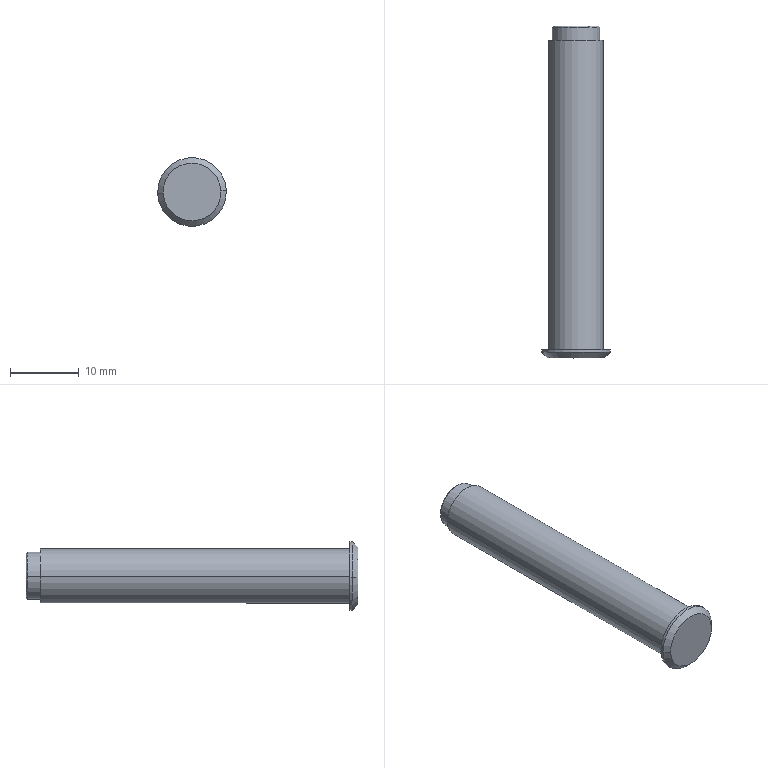Part | SolidWorks | features BaseBody 1 | 1 solid | 17 faces | box 10 x 48.303 x 10 mm | volume 2156 mm3 | cylinder 8 | plane 5 | cone 4 | commonest cylinder face diameters 5.2 x2 6.9 x2 7.9 x2 10 x2
STEP:
#1=CARTESIAN_POINT('',(-215.071,6.123,1.995));
#2=VERTEX_POINT('',#1);
#3=CARTESIAN_POINT('',(-209.875,6.123,2.179));
#4=VERTEX_POINT('',#3);
#5=CARTESIAN_POINT('',(-212.473,6.123,2.087));
#6=DIRECTION('',(0.00003827,-1.,-0.0004455));
#7=DIRECTION('',(-0.9994,-0.0000225,-0.03534));
#8=AXIS2_PLACEMENT_3D('',#5,#6,#7);
#9=CIRCLE('',#8,2.6);
#10=EDGE_CURVE('',#2,#4,#9,.T.);
#11=ORIENTED_EDGE('',*,*,#10,.F.);
#12=CARTESIAN_POINT('',(-212.473,6.123,2.087));
#13=DIRECTION('',(0.00003827,-1.,-0.0004455));
#14=DIRECTION('',(0.9994,0.0000225,0.03534));
#15=AXIS2_PLACEMENT_3D('',#12,#13,#14);
#16=CIRCLE('',#15,2.6);
#17=EDGE_CURVE('',#4,#2,#16,.T.);
#18=ORIENTED_EDGE('',*,*,#17,.F.);
#19=EDGE_LOOP('',(#11,#18));
#20=FACE_OUTER_BOUND('',#19,.T.);
#21=CARTESIAN_POINT('',(-212.473,6.123,2.087));
#22=DIRECTION('',(-0.00003827,1.,0.0004455));
#23=DIRECTION('',(0.9963,0.,0.08559));
#24=AXIS2_PLACEMENT_3D('',#21,#22,#23);
#25=PLANE('',#24);
#26=ADVANCED_FACE('',(#20),#25,.T.);
#27=ORIENTED_EDGE('',*,*,#17,.T.);
#28=CARTESIAN_POINT('',(-215.072,16.123,2.));
#29=VERTEX_POINT('',#28);
#30=CARTESIAN_POINT('',(-215.072,16.123,2.));
#31=DIRECTION('',(0.00003827,-1.,-0.0004455));
#32=VECTOR('',#31,1000.);
#33=LINE('',#30,#32);
#34=EDGE_CURVE('',#29,#2,#33,.T.);
#35=ORIENTED_EDGE('',*,*,#34,.F.);
#36=CARTESIAN_POINT('',(-209.875,16.123,2.183));
#37=VERTEX_POINT('',#36);
#38=CARTESIAN_POINT('',(-212.473,16.123,2.092));
#39=DIRECTION('',(-0.00003827,1.,0.0004455));
#40=DIRECTION('',(-0.9994,-0.0000225,-0.03534));
#41=AXIS2_PLACEMENT_3D('',#38,#39,#40);
#42=CIRCLE('',#41,2.6);
#43=EDGE_CURVE('',#29,#37,#42,.T.);
#44=ORIENTED_EDGE('',*,*,#43,.T.);
#45=CARTESIAN_POINT('',(-209.875,16.123,2.183));
#46=DIRECTION('',(0.00003827,-1.,-0.0004455));
#47=VECTOR('',#46,1000.);
#48=LINE('',#45,#47);
#49=EDGE_CURVE('',#37,#4,#48,.T.);
#50=ORIENTED_EDGE('',*,*,#49,.T.);
#51=EDGE_LOOP('',(#27,#35,#44,#50));
#52=FACE_OUTER_BOUND('',#51,.T.);
#53=CARTESIAN_POINT('',(-212.473,6.123,2.087));
#54=DIRECTION('',(-0.00003827,1.,0.0004455));
#55=DIRECTION('',(-0.9994,-0.0000225,-0.03534));
#56=AXIS2_PLACEMENT_3D('',#53,#54,#55);
#57=CYLINDRICAL_SURFACE('',#56,2.6);
#58=ADVANCED_FACE('',(#52),#57,.F.);
#59=ORIENTED_EDGE('',*,*,#49,.F.);
#60=CARTESIAN_POINT('',(-212.473,16.123,2.092));
#61=DIRECTION('',(-0.00003827,1.,0.0004455));
#62=DIRECTION('',(0.9994,0.0000225,0.03534));
#63=AXIS2_PLACEMENT_3D('',#60,#61,#62);
#64=CIRCLE('',#63,2.6);
#65=EDGE_CURVE('',#37,#29,#64,.T.);
#66=ORIENTED_EDGE('',*,*,#65,.T.);
#67=ORIENTED_EDGE('',*,*,#34,.T.);
#68=ORIENTED_EDGE('',*,*,#10,.T.);
#69=EDGE_LOOP('',(#59,#66,#67,#68));
#70=FACE_OUTER_BOUND('',#69,.T.);
#71=CARTESIAN_POINT('',(-212.473,6.123,2.087));
#72=DIRECTION('',(-0.00003827,1.,0.0004455));
#73=DIRECTION('',(-0.9994,-0.0000225,-0.03534));
#74=AXIS2_PLACEMENT_3D('',#71,#72,#73);
#75=CYLINDRICAL_SURFACE('',#74,2.6);
#76=ADVANCED_FACE('',(#70),#75,.F.);
#77=ORIENTED_EDGE('',*,*,#65,.F.);
#78=ORIENTED_EDGE('',*,*,#43,.F.);
#79=EDGE_LOOP('',(#77,#78));
#80=FACE_BOUND('',#79,.T.);
#81=CARTESIAN_POINT('',(-209.225,16.123,2.206));
#82=VERTEX_POINT('',#81);
#83=CARTESIAN_POINT('',(-215.721,16.123,1.977));
#84=VERTEX_POINT('',#83);
#85=CARTESIAN_POINT('',(-212.473,16.123,2.092));
#86=DIRECTION('',(0.00003827,-1.,-0.0004455));
#87=DIRECTION('',(0.9994,0.0000225,0.03534));
#88=AXIS2_PLACEMENT_3D('',#85,#86,#87);
#89=CIRCLE('',#88,3.25);
#90=EDGE_CURVE('',#82,#84,#89,.T.);
#91=ORIENTED_EDGE('',*,*,#90,.F.);
#92=CARTESIAN_POINT('',(-212.473,16.123,2.092));
#93=DIRECTION('',(0.00003827,-1.,-0.0004455));
#94=DIRECTION('',(-0.9994,-0.0000225,-0.03534));
#95=AXIS2_PLACEMENT_3D('',#92,#93,#94);
#96=CIRCLE('',#95,3.25);
#97=EDGE_CURVE('',#84,#82,#96,.T.);
#98=ORIENTED_EDGE('',*,*,#97,.F.);
#99=EDGE_LOOP('',(#91,#98));
#100=FACE_OUTER_BOUND('',#99,.T.);
#101=CARTESIAN_POINT('',(-212.473,16.123,2.092));
#102=DIRECTION('',(-0.00003827,1.,0.0004455));
#103=DIRECTION('',(0.9963,0.,0.08559));
#104=AXIS2_PLACEMENT_3D('',#101,#102,#103);
#105=PLANE('',#104);
#106=ADVANCED_FACE('',(#80,#100),#105,.T.);
#107=ORIENTED_EDGE('',*,*,#97,.T.);
#108=CARTESIAN_POINT('',(-209.025,15.923,2.213));
#109=VERTEX_POINT('',#108);
#110=CARTESIAN_POINT('',(-209.025,15.923,2.213));
#111=DIRECTION('',(-0.7067,0.7071,-0.02468));
#112=VECTOR('',#111,1000.);
#113=LINE('',#110,#112);
#114=EDGE_CURVE('',#109,#82,#113,.T.);
#115=ORIENTED_EDGE('',*,*,#114,.F.);
#116=CARTESIAN_POINT('',(-215.921,15.923,1.97));
#117=VERTEX_POINT('',#116);
#118=CARTESIAN_POINT('',(-212.473,15.923,2.091));
#119=DIRECTION('',(0.00003827,-1.,-0.0004455));
#120=DIRECTION('',(-0.9994,-0.0000225,-0.03534));
#121=AXIS2_PLACEMENT_3D('',#118,#119,#120);
#122=CIRCLE('',#121,3.45);
#123=EDGE_CURVE('',#117,#109,#122,.T.);
#124=ORIENTED_EDGE('',*,*,#123,.F.);
#125=CARTESIAN_POINT('',(-215.921,15.923,1.97));
#126=DIRECTION('',(0.7066,0.7071,0.02531));
#127=VECTOR('',#126,1000.);
#128=LINE('',#125,#127);
#129=EDGE_CURVE('',#117,#84,#128,.T.);
#130=ORIENTED_EDGE('',*,*,#129,.T.);
#131=EDGE_LOOP('',(#107,#115,#124,#130));
#132=FACE_OUTER_BOUND('',#131,.T.);
#133=CARTESIAN_POINT('',(-212.473,16.023,2.092));
#134=DIRECTION('',(0.00003827,-1.,-0.0004455));
#135=DIRECTION('',(0.9994,0.0000225,0.03534));
#136=AXIS2_PLACEMENT_3D('',#133,#134,#135);
#137=CONICAL_SURFACE('',#136,3.35,0.7854);
#138=ADVANCED_FACE('',(#132),#137,.T.);
#139=ORIENTED_EDGE('',*,*,#129,.F.);
#140=CARTESIAN_POINT('',(-212.473,15.923,2.091));
#141=DIRECTION('',(0.00003827,-1.,-0.0004455));
#142=DIRECTION('',(0.9994,0.0000225,0.03534));
#143=AXIS2_PLACEMENT_3D('',#140,#141,#142);
#144=CIRCLE('',#143,3.45);
#145=EDGE_CURVE('',#109,#117,#144,.T.);
#146=ORIENTED_EDGE('',*,*,#145,.F.);
#147=ORIENTED_EDGE('',*,*,#114,.T.);
#148=ORIENTED_EDGE('',*,*,#90,.T.);
#149=EDGE_LOOP('',(#139,#146,#147,#148));
#150=FACE_OUTER_BOUND('',#149,.T.);
#151=CARTESIAN_POINT('',(-212.473,16.023,2.092));
#152=DIRECTION('',(0.00003827,-1.,-0.0004455));
#153=DIRECTION('',(0.9994,0.0000225,0.03534));
#154=AXIS2_PLACEMENT_3D('',#151,#152,#153);
#155=CONICAL_SURFACE('',#154,3.35,0.7854);
#156=ADVANCED_FACE('',(#150),#155,.T.);
#157=CARTESIAN_POINT('',(-215.921,14.023,1.969));
#158=VERTEX_POINT('',#157);
#159=CARTESIAN_POINT('',(-215.921,14.023,1.969));
#160=DIRECTION('',(-0.00003827,1.,0.0004455));
#161=VECTOR('',#160,1000.);
#162=LINE('',#159,#161);
#163=EDGE_CURVE('',#158,#117,#162,.T.);
#164=ORIENTED_EDGE('',*,*,#163,.F.);
#165=CARTESIAN_POINT('',(-209.025,14.023,2.213));
#166=VERTEX_POINT('',#165);
#167=CARTESIAN_POINT('',(-212.473,14.023,2.091));
#168=DIRECTION('',(-0.00003827,1.,0.0004455));
#169=DIRECTION('',(-0.9994,-0.0000225,-0.03534));
#170=AXIS2_PLACEMENT_3D('',#167,#168,#169);
#171=CIRCLE('',#170,3.45);
#172=EDGE_CURVE('',#158,#166,#171,.T.);
#173=ORIENTED_EDGE('',*,*,#172,.T.);
#174=CARTESIAN_POINT('',(-209.025,14.023,2.213));
#175=DIRECTION('',(-0.00003827,1.,0.0004455));
#176=VECTOR('',#175,1000.);
#177=LINE('',#174,#176);
#178=EDGE_CURVE('',#166,#109,#177,.T.);
#179=ORIENTED_EDGE('',*,*,#178,.T.);
#180=ORIENTED_EDGE('',*,*,#145,.T.);
#181=EDGE_LOOP('',(#164,#173,#179,#180));
#182=FACE_OUTER_BOUND('',#181,.T.);
#183=CARTESIAN_POINT('',(-212.473,16.123,2.092));
#184=DIRECTION('',(0.00003827,-1.,-0.0004455));
#185=DIRECTION('',(0.9994,0.0000225,0.03534));
#186=AXIS2_PLACEMENT_3D('',#183,#184,#185);
#187=CYLINDRICAL_SURFACE('',#186,3.45);
#188=ADVANCED_FACE('',(#182),#187,.T.);
#189=ORIENTED_EDGE('',*,*,#123,.T.);
#190=ORIENTED_EDGE('',*,*,#178,.F.);
#191=CARTESIAN_POINT('',(-212.473,14.023,2.091));
#192=DIRECTION('',(-0.00003827,1.,0.0004455));
#193=DIRECTION('',(0.9994,0.0000225,0.03534));
#194=AXIS2_PLACEMENT_3D('',#191,#192,#193);
#195=CIRCLE('',#194,3.45);
#196=EDGE_CURVE('',#166,#158,#195,.T.);
#197=ORIENTED_EDGE('',*,*,#196,.T.);
#198=ORIENTED_EDGE('',*,*,#163,.T.);
#199=EDGE_LOOP('',(#189,#190,#197,#198));
#200=FACE_OUTER_BOUND('',#199,.T.);
#201=CARTESIAN_POINT('',(-212.473,16.123,2.092));
#202=DIRECTION('',(0.00003827,-1.,-0.0004455));
#203=DIRECTION('',(0.9994,0.0000225,0.03534));
#204=AXIS2_PLACEMENT_3D('',#201,#202,#203);
#205=CYLINDRICAL_SURFACE('',#204,3.45);
#206=ADVANCED_FACE('',(#200),#205,.T.);
#207=ORIENTED_EDGE('',*,*,#172,.F.);
#208=ORIENTED_EDGE('',*,*,#196,.F.);
#209=EDGE_LOOP('',(#207,#208));
#210=FACE_BOUND('',#209,.T.);
#211=CARTESIAN_POINT('',(-208.526,14.023,2.23));
#212=VERTEX_POINT('',#211);
#213=CARTESIAN_POINT('',(-216.421,14.023,1.951));
#214=VERTEX_POINT('',#213);
#215=CARTESIAN_POINT('',(-212.473,14.023,2.091));
#216=DIRECTION('',(0.00003827,-1.,-0.0004455));
#217=DIRECTION('',(0.9994,0.0000225,0.03534));
#218=AXIS2_PLACEMENT_3D('',#215,#216,#217);
#219=CIRCLE('',#218,3.95);
#220=EDGE_CURVE('',#212,#214,#219,.T.);
#221=ORIENTED_EDGE('',*,*,#220,.F.);
#222=CARTESIAN_POINT('',(-212.473,14.023,2.091));
#223=DIRECTION('',(0.00003827,-1.,-0.0004455));
#224=DIRECTION('',(-0.9994,-0.0000225,-0.03534));
#225=AXIS2_PLACEMENT_3D('',#222,#223,#224);
#226=CIRCLE('',#225,3.95);
#227=EDGE_CURVE('',#214,#212,#226,.T.);
#228=ORIENTED_EDGE('',*,*,#227,.F.);
#229=EDGE_LOOP('',(#221,#228));
#230=FACE_OUTER_BOUND('',#229,.T.);
#231=CARTESIAN_POINT('',(-212.473,14.023,2.091));
#232=DIRECTION('',(-0.00003827,1.,0.0004455));
#233=DIRECTION('',(0.9963,0.,0.08559));
#234=AXIS2_PLACEMENT_3D('',#231,#232,#233);
#235=PLANE('',#234);
#236=ADVANCED_FACE('',(#210,#230),#235,.T.);
#237=ORIENTED_EDGE('',*,*,#227,.T.);
#238=CARTESIAN_POINT('',(-208.524,-30.977,2.21));
#239=VERTEX_POINT('',#238);
#240=CARTESIAN_POINT('',(-208.524,-30.977,2.21));
#241=DIRECTION('',(-0.00003827,1.,0.0004455));
#242=VECTOR('',#241,1000.);
#243=LINE('',#240,#242);
#244=EDGE_CURVE('',#239,#212,#243,.T.);
#245=ORIENTED_EDGE('',*,*,#244,.F.);
#246=CARTESIAN_POINT('',(-216.419,-30.977,1.931));
#247=VERTEX_POINT('',#246);
#248=CARTESIAN_POINT('',(-212.472,-30.977,2.071));
#249=DIRECTION('',(-0.00003827,1.,0.0004455));
#250=DIRECTION('',(0.9994,0.0000225,0.03534));
#251=AXIS2_PLACEMENT_3D('',#248,#249,#250);
#252=CIRCLE('',#251,3.95);
#253=EDGE_CURVE('',#239,#247,#252,.T.);
#254=ORIENTED_EDGE('',*,*,#253,.T.);
#255=CARTESIAN_POINT('',(-216.419,-30.977,1.931));
#256=DIRECTION('',(-0.00003827,1.,0.0004455));
#257=VECTOR('',#256,1000.);
#258=LINE('',#255,#257);
#259=EDGE_CURVE('',#247,#214,#258,.T.);
#260=ORIENTED_EDGE('',*,*,#259,.T.);
#261=EDGE_LOOP('',(#237,#245,#254,#260));
#262=FACE_OUTER_BOUND('',#261,.T.);
#263=CARTESIAN_POINT('',(-212.473,14.023,2.091));
#264=DIRECTION('',(0.00003827,-1.,-0.0004455));
#265=DIRECTION('',(0.9994,0.0000225,0.03534));
#266=AXIS2_PLACEMENT_3D('',#263,#264,#265);
#267=CYLINDRICAL_SURFACE('',#266,3.95);
#268=ADVANCED_FACE('',(#262),#267,.T.);
#269=ORIENTED_EDGE('',*,*,#259,.F.);
#270=CARTESIAN_POINT('',(-212.472,-30.977,2.071));
#271=DIRECTION('',(-0.00003827,1.,0.0004455));
#272=DIRECTION('',(-0.9994,-0.0000225,-0.03534));
#273=AXIS2_PLACEMENT_3D('',#270,#271,#272);
#274=CIRCLE('',#273,3.95);
#275=EDGE_CURVE('',#247,#239,#274,.T.);
#276=ORIENTED_EDGE('',*,*,#275,.T.);
#277=ORIENTED_EDGE('',*,*,#244,.T.);
#278=ORIENTED_EDGE('',*,*,#220,.T.);
#279=EDGE_LOOP('',(#269,#276,#277,#278));
#280=FACE_OUTER_BOUND('',#279,.T.);
#281=CARTESIAN_POINT('',(-212.473,14.023,2.091));
#282=DIRECTION('',(0.00003827,-1.,-0.0004455));
#283=DIRECTION('',(0.9994,0.0000225,0.03534));
#284=AXIS2_PLACEMENT_3D('',#281,#282,#283);
#285=CYLINDRICAL_SURFACE('',#284,3.95);
#286=ADVANCED_FACE('',(#280),#285,.T.);
#287=ORIENTED_EDGE('',*,*,#275,.F.);
#288=ORIENTED_EDGE('',*,*,#253,.F.);
#289=EDGE_LOOP('',(#287,#288));
#290=FACE_BOUND('',#289,.T.);
#291=CARTESIAN_POINT('',(-207.475,-30.977,2.247));
#292=VERTEX_POINT('',#291);
#293=CARTESIAN_POINT('',(-217.468,-30.977,1.894));
#294=VERTEX_POINT('',#293);
#295=CARTESIAN_POINT('',(-212.472,-30.977,2.071));
#296=DIRECTION('',(0.00003827,-1.,-0.0004455));
#297=DIRECTION('',(0.9994,0.0000225,0.03534));
#298=AXIS2_PLACEMENT_3D('',#295,#296,#297);
#299=CIRCLE('',#298,5.);
#300=EDGE_CURVE('',#292,#294,#299,.T.);
#301=ORIENTED_EDGE('',*,*,#300,.F.);
#302=CARTESIAN_POINT('',(-212.472,-30.977,2.071));
#303=DIRECTION('',(0.00003827,-1.,-0.0004455));
#304=DIRECTION('',(-0.9994,-0.0000225,-0.03534));
#305=AXIS2_PLACEMENT_3D('',#302,#303,#304);
#306=CIRCLE('',#305,5.);
#307=EDGE_CURVE('',#294,#292,#306,.T.);
#308=ORIENTED_EDGE('',*,*,#307,.F.);
#309=EDGE_LOOP('',(#301,#308));
#310=FACE_OUTER_BOUND('',#309,.T.);
#311=CARTESIAN_POINT('',(-212.472,-30.977,2.071));
#312=DIRECTION('',(-0.00003827,1.,0.0004455));
#313=DIRECTION('',(0.9963,0.,0.08559));
#314=AXIS2_PLACEMENT_3D('',#311,#312,#313);
#315=PLANE('',#314);
#316=ADVANCED_FACE('',(#290,#310),#315,.T.);
#317=ORIENTED_EDGE('',*,*,#307,.T.);
#318=CARTESIAN_POINT('',(-207.475,-31.377,2.247));
#319=VERTEX_POINT('',#318);
#320=CARTESIAN_POINT('',(-207.475,-31.377,2.247));
#321=DIRECTION('',(-0.00003827,1.,0.0004455));
#322=VECTOR('',#321,1000.);
#323=LINE('',#320,#322);
#324=EDGE_CURVE('',#319,#292,#323,.T.);
#325=ORIENTED_EDGE('',*,*,#324,.F.);
#326=CARTESIAN_POINT('',(-217.468,-31.377,1.894));
#327=VERTEX_POINT('',#326);
#328=CARTESIAN_POINT('',(-212.471,-31.377,2.07));
#329=DIRECTION('',(-0.00003827,1.,0.0004455));
#330=DIRECTION('',(0.9994,0.0000225,0.03534));
#331=AXIS2_PLACEMENT_3D('',#328,#329,#330);
#332=CIRCLE('',#331,5.);
#333=EDGE_CURVE('',#319,#327,#332,.T.);
#334=ORIENTED_EDGE('',*,*,#333,.T.);
#335=CARTESIAN_POINT('',(-217.468,-31.377,1.894));
#336=DIRECTION('',(-0.00003827,1.,0.0004455));
#337=VECTOR('',#336,1000.);
#338=LINE('',#335,#337);
#339=EDGE_CURVE('',#327,#294,#338,.T.);
#340=ORIENTED_EDGE('',*,*,#339,.T.);
#341=EDGE_LOOP('',(#317,#325,#334,#340));
#342=FACE_OUTER_BOUND('',#341,.T.);
#343=CARTESIAN_POINT('',(-212.472,-30.977,2.071));
#344=DIRECTION('',(0.00003827,-1.,-0.0004455));
#345=DIRECTION('',(0.9994,0.0000225,0.03534));
#346=AXIS2_PLACEMENT_3D('',#343,#344,#345);
#347=CYLINDRICAL_SURFACE('',#346,5.);
#348=ADVANCED_FACE('',(#342),#347,.T.);
#349=ORIENTED_EDGE('',*,*,#339,.F.);
#350=CARTESIAN_POINT('',(-212.471,-31.377,2.07));
#351=DIRECTION('',(-0.00003827,1.,0.0004455));
#352=DIRECTION('',(-0.9994,-0.0000225,-0.03534));
#353=AXIS2_PLACEMENT_3D('',#350,#351,#352);
#354=CIRCLE('',#353,5.);
#355=EDGE_CURVE('',#327,#319,#354,.T.);
#356=ORIENTED_EDGE('',*,*,#355,.T.);
#357=ORIENTED_EDGE('',*,*,#324,.T.);
#358=ORIENTED_EDGE('',*,*,#300,.T.);
#359=EDGE_LOOP('',(#349,#356,#357,#358));
#360=FACE_OUTER_BOUND('',#359,.T.);
#361=CARTESIAN_POINT('',(-212.472,-30.977,2.071));
#362=DIRECTION('',(0.00003827,-1.,-0.0004455));
#363=DIRECTION('',(0.9994,0.0000225,0.03534));
#364=AXIS2_PLACEMENT_3D('',#361,#362,#363);
#365=CYLINDRICAL_SURFACE('',#364,5.);
#366=ADVANCED_FACE('',(#360),#365,.T.);
#367=CARTESIAN_POINT('',(-208.274,-32.177,2.218));
#368=VERTEX_POINT('',#367);
#369=CARTESIAN_POINT('',(-207.475,-31.377,2.247));
#370=DIRECTION('',(-0.7066,-0.7071,-0.02531));
#371=VECTOR('',#370,1000.);
#372=LINE('',#369,#371);
#373=EDGE_CURVE('',#319,#368,#372,.T.);
#374=ORIENTED_EDGE('',*,*,#373,.F.);
#375=ORIENTED_EDGE('',*,*,#355,.F.);
#376=CARTESIAN_POINT('',(-216.669,-32.177,1.922));
#377=VERTEX_POINT('',#376);
#378=CARTESIAN_POINT('',(-217.468,-31.377,1.894));
#379=DIRECTION('',(0.7067,-0.7071,0.02468));
#380=VECTOR('',#379,1000.);
#381=LINE('',#378,#380);
#382=EDGE_CURVE('',#327,#377,#381,.T.);
#383=ORIENTED_EDGE('',*,*,#382,.T.);
#384=CARTESIAN_POINT('',(-212.471,-32.177,2.07));
#385=DIRECTION('',(-0.00003827,1.,0.0004455));
#386=DIRECTION('',(-0.9994,-0.0000225,-0.03534));
#387=AXIS2_PLACEMENT_3D('',#384,#385,#386);
#388=CIRCLE('',#387,4.2);
#389=EDGE_CURVE('',#377,#368,#388,.T.);
#390=ORIENTED_EDGE('',*,*,#389,.T.);
#391=EDGE_LOOP('',(#374,#375,#383,#390));
#392=FACE_OUTER_BOUND('',#391,.T.);
#393=CARTESIAN_POINT('',(-212.471,-31.777,2.07));
#394=DIRECTION('',(-0.00003827,1.,0.0004455));
#395=DIRECTION('',(-0.9994,-0.0000225,-0.03534));
#396=AXIS2_PLACEMENT_3D('',#393,#394,#395);
#397=CONICAL_SURFACE('',#396,4.6,0.7854);
#398=ADVANCED_FACE('',(#392),#397,.T.);
#399=ORIENTED_EDGE('',*,*,#389,.F.);
#400=CARTESIAN_POINT('',(-212.471,-32.177,2.07));
#401=DIRECTION('',(-0.00003827,1.,0.0004455));
#402=DIRECTION('',(0.9994,0.0000225,0.03534));
#403=AXIS2_PLACEMENT_3D('',#400,#401,#402);
#404=CIRCLE('',#403,4.2);
#405=EDGE_CURVE('',#368,#377,#404,.T.);
#406=ORIENTED_EDGE('',*,*,#405,.F.);
#407=EDGE_LOOP('',(#399,#406));
#408=FACE_OUTER_BOUND('',#407,.T.);
#409=CARTESIAN_POINT('',(-212.471,-32.177,2.07));
#410=DIRECTION('',(-0.00003827,1.,0.0004455));
#411=DIRECTION('',(0.9963,0.,0.08559));
#412=AXIS2_PLACEMENT_3D('',#409,#410,#411);
#413=PLANE('',#412);
#414=ADVANCED_FACE('',(#408),#413,.F.);
#415=ORIENTED_EDGE('',*,*,#405,.T.);
#416=ORIENTED_EDGE('',*,*,#382,.F.);
#417=ORIENTED_EDGE('',*,*,#333,.F.);
#418=ORIENTED_EDGE('',*,*,#373,.T.);
#419=EDGE_LOOP('',(#415,#416,#417,#418));
#420=FACE_OUTER_BOUND('',#419,.T.);
#421=CARTESIAN_POINT('',(-212.471,-31.777,2.07));
#422=DIRECTION('',(-0.00003827,1.,0.0004455));
#423=DIRECTION('',(-0.9994,-0.0000225,-0.03534));
#424=AXIS2_PLACEMENT_3D('',#421,#422,#423);
#425=CONICAL_SURFACE('',#424,4.6,0.7854);
#426=ADVANCED_FACE('',(#420),#425,.T.);
#427=CLOSED_SHELL('',(#26,#58,#76,#106,#138,#156,#188,#206,#236,#268,#286,#316,#348,#366,#398,#414,#426));
#428=MANIFOLD_SOLID_BREP('',#427);
#429=CARTESIAN_POINT('',(0.,0.,0.));
#430=DIRECTION('',(0.,0.,1.));
#431=DIRECTION('',(1.,0.,0.));
#432=AXIS2_PLACEMENT_3D('',#429,#430,#431);
#433=(LENGTH_UNIT()NAMED_UNIT(*)SI_UNIT(.MILLI.,.METRE.));
#434=UNCERTAINTY_MEASURE_WITH_UNIT(LENGTH_MEASURE(0.00001),#433,'','');
#435=(NAMED_UNIT(*)PLANE_ANGLE_UNIT()SI_UNIT($,.RADIAN.));
#436=(NAMED_UNIT(*)SI_UNIT($,.STERADIAN.)SOLID_ANGLE_UNIT());
#437=(GEOMETRIC_REPRESENTATION_CONTEXT(3)GLOBAL_UNCERTAINTY_ASSIGNED_CONTEXT((#434))GLOBAL_UNIT_ASSIGNED_CONTEXT((#433,#435,#436))REPRESENTATION_CONTEXT('',''));
#438=ADVANCED_BREP_SHAPE_REPRESENTATION('',(#428,#432),#437);